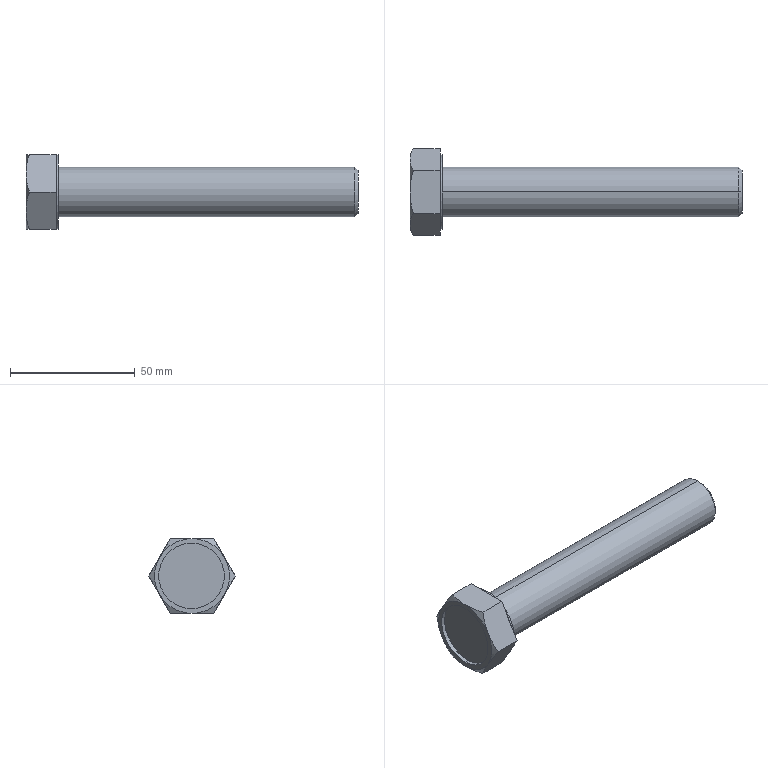Part | STEP file | formed hex screw_am_B18.2.3.2M - Formed hex screw, M20 x 2.5 x 120 --46WN | 1 solid | 30 faces | box 132.88 x 34.641 x 30 mm | volume 46723 mm3 | plane 16 | cone 8 | cylinder 6 | commonest cylinder face diameters 20 x2 26.25 x2 30 x2